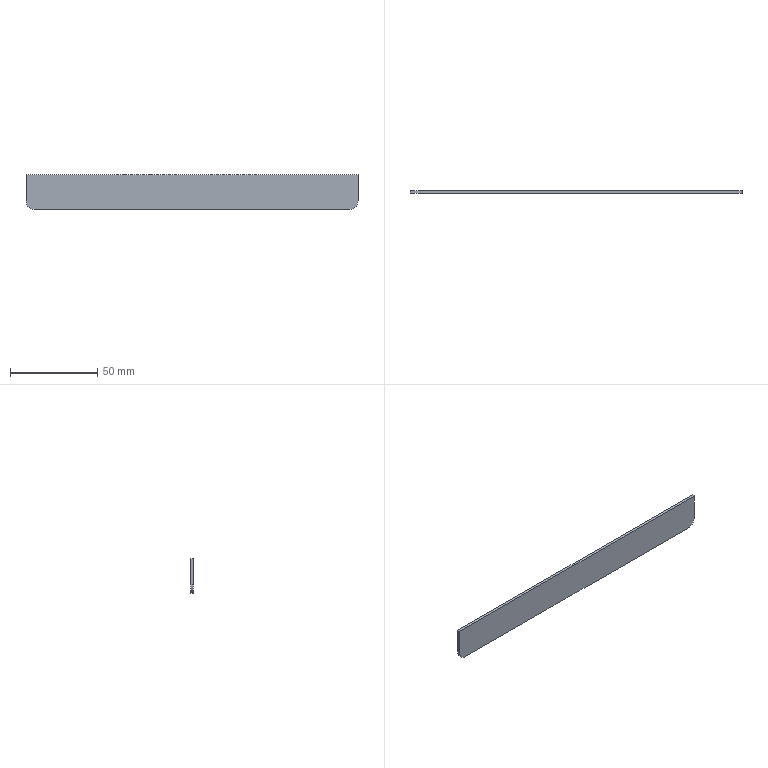Part | SolidWorks | features Extrusion 1 | 1 solid | 8 faces | box 190 x 1.6 x 20 mm | volume 6063 mm3 | plane 6 | cylinder 2 | commonest cylinder face diameters 10 x2
STEP:
#1=CARTESIAN_POINT('',(0.,0.,-15.));
#2=VERTEX_POINT('',#1);
#3=CARTESIAN_POINT('',(0.,0.,0.));
#4=VERTEX_POINT('',#3);
#5=CARTESIAN_POINT('',(0.,0.,0.));
#6=DIRECTION('',(0.,0.,1.));
#7=VECTOR('',#6,1000.);
#8=LINE('',#5,#7);
#9=EDGE_CURVE('',#2,#4,#8,.T.);
#10=ORIENTED_EDGE('',*,*,#9,.T.);
#11=CARTESIAN_POINT('',(0.,1.6,0.));
#12=VERTEX_POINT('',#11);
#13=CARTESIAN_POINT('',(0.,1.6,0.));
#14=DIRECTION('',(0.,-1.,0.));
#15=VECTOR('',#14,1000.);
#16=LINE('',#13,#15);
#17=EDGE_CURVE('',#12,#4,#16,.T.);
#18=ORIENTED_EDGE('',*,*,#17,.F.);
#19=CARTESIAN_POINT('',(0.,1.6,-15.));
#20=VERTEX_POINT('',#19);
#21=CARTESIAN_POINT('',(0.,1.6,0.));
#22=DIRECTION('',(0.,0.,1.));
#23=VECTOR('',#22,1000.);
#24=LINE('',#21,#23);
#25=EDGE_CURVE('',#20,#12,#24,.T.);
#26=ORIENTED_EDGE('',*,*,#25,.F.);
#27=CARTESIAN_POINT('',(0.,1.6,-15.));
#28=DIRECTION('',(0.,-1.,0.));
#29=VECTOR('',#28,1000.);
#30=LINE('',#27,#29);
#31=EDGE_CURVE('',#20,#2,#30,.T.);
#32=ORIENTED_EDGE('',*,*,#31,.T.);
#33=EDGE_LOOP('',(#10,#18,#26,#32));
#34=FACE_OUTER_BOUND('',#33,.T.);
#35=CARTESIAN_POINT('',(0.,1.6,0.));
#36=DIRECTION('',(1.,0.,0.));
#37=DIRECTION('',(0.,0.,-1.));
#38=AXIS2_PLACEMENT_3D('',#35,#36,#37);
#39=PLANE('',#38);
#40=ADVANCED_FACE('',(#34),#39,.F.);
#41=CARTESIAN_POINT('',(190.,0.,0.));
#42=VERTEX_POINT('',#41);
#43=CARTESIAN_POINT('',(0.,0.,0.));
#44=DIRECTION('',(1.,0.,0.));
#45=VECTOR('',#44,1000.);
#46=LINE('',#43,#45);
#47=EDGE_CURVE('',#4,#42,#46,.T.);
#48=ORIENTED_EDGE('',*,*,#47,.T.);
#49=CARTESIAN_POINT('',(190.,1.6,0.));
#50=VERTEX_POINT('',#49);
#51=CARTESIAN_POINT('',(190.,1.6,0.));
#52=DIRECTION('',(0.,-1.,0.));
#53=VECTOR('',#52,1000.);
#54=LINE('',#51,#53);
#55=EDGE_CURVE('',#50,#42,#54,.T.);
#56=ORIENTED_EDGE('',*,*,#55,.F.);
#57=CARTESIAN_POINT('',(0.,1.6,0.));
#58=DIRECTION('',(1.,0.,0.));
#59=VECTOR('',#58,1000.);
#60=LINE('',#57,#59);
#61=EDGE_CURVE('',#12,#50,#60,.T.);
#62=ORIENTED_EDGE('',*,*,#61,.F.);
#63=ORIENTED_EDGE('',*,*,#17,.T.);
#64=EDGE_LOOP('',(#48,#56,#62,#63));
#65=FACE_OUTER_BOUND('',#64,.T.);
#66=CARTESIAN_POINT('',(0.,1.6,0.));
#67=DIRECTION('',(0.,0.,-1.));
#68=DIRECTION('',(-1.,0.,0.));
#69=AXIS2_PLACEMENT_3D('',#66,#67,#68);
#70=PLANE('',#69);
#71=ADVANCED_FACE('',(#65),#70,.F.);
#72=CARTESIAN_POINT('',(190.,0.,-15.));
#73=VERTEX_POINT('',#72);
#74=CARTESIAN_POINT('',(190.,0.,0.));
#75=DIRECTION('',(0.,0.,-1.));
#76=VECTOR('',#75,1000.);
#77=LINE('',#74,#76);
#78=EDGE_CURVE('',#42,#73,#77,.T.);
#79=ORIENTED_EDGE('',*,*,#78,.T.);
#80=CARTESIAN_POINT('',(190.,1.6,-15.));
#81=VERTEX_POINT('',#80);
#82=CARTESIAN_POINT('',(190.,1.6,-15.));
#83=DIRECTION('',(0.,-1.,0.));
#84=VECTOR('',#83,1000.);
#85=LINE('',#82,#84);
#86=EDGE_CURVE('',#81,#73,#85,.T.);
#87=ORIENTED_EDGE('',*,*,#86,.F.);
#88=CARTESIAN_POINT('',(190.,1.6,0.));
#89=DIRECTION('',(0.,0.,-1.));
#90=VECTOR('',#89,1000.);
#91=LINE('',#88,#90);
#92=EDGE_CURVE('',#50,#81,#91,.T.);
#93=ORIENTED_EDGE('',*,*,#92,.F.);
#94=ORIENTED_EDGE('',*,*,#55,.T.);
#95=EDGE_LOOP('',(#79,#87,#93,#94));
#96=FACE_OUTER_BOUND('',#95,.T.);
#97=CARTESIAN_POINT('',(190.,1.6,0.));
#98=DIRECTION('',(-1.,0.,0.));
#99=DIRECTION('',(0.,0.,1.));
#100=AXIS2_PLACEMENT_3D('',#97,#98,#99);
#101=PLANE('',#100);
#102=ADVANCED_FACE('',(#96),#101,.F.);
#103=CARTESIAN_POINT('',(185.,0.,-20.));
#104=VERTEX_POINT('',#103);
#105=CARTESIAN_POINT('',(185.,0.,-15.));
#106=DIRECTION('',(0.,1.,0.));
#107=DIRECTION('',(0.,0.,-1.));
#108=AXIS2_PLACEMENT_3D('',#105,#106,#107);
#109=CIRCLE('',#108,5.);
#110=EDGE_CURVE('',#73,#104,#109,.T.);
#111=ORIENTED_EDGE('',*,*,#110,.T.);
#112=CARTESIAN_POINT('',(185.,1.6,-20.));
#113=VERTEX_POINT('',#112);
#114=CARTESIAN_POINT('',(185.,1.6,-20.));
#115=DIRECTION('',(0.,-1.,0.));
#116=VECTOR('',#115,1000.);
#117=LINE('',#114,#116);
#118=EDGE_CURVE('',#113,#104,#117,.T.);
#119=ORIENTED_EDGE('',*,*,#118,.F.);
#120=CARTESIAN_POINT('',(185.,1.6,-15.));
#121=DIRECTION('',(0.,1.,0.));
#122=DIRECTION('',(0.,0.,-1.));
#123=AXIS2_PLACEMENT_3D('',#120,#121,#122);
#124=CIRCLE('',#123,5.);
#125=EDGE_CURVE('',#81,#113,#124,.T.);
#126=ORIENTED_EDGE('',*,*,#125,.F.);
#127=ORIENTED_EDGE('',*,*,#86,.T.);
#128=EDGE_LOOP('',(#111,#119,#126,#127));
#129=FACE_OUTER_BOUND('',#128,.T.);
#130=CARTESIAN_POINT('',(185.,1.6,-15.));
#131=DIRECTION('',(0.,-1.,0.));
#132=DIRECTION('',(0.,0.,-1.));
#133=AXIS2_PLACEMENT_3D('',#130,#131,#132);
#134=CYLINDRICAL_SURFACE('',#133,5.);
#135=ADVANCED_FACE('',(#129),#134,.T.);
#136=CARTESIAN_POINT('',(5.,0.,-20.));
#137=VERTEX_POINT('',#136);
#138=CARTESIAN_POINT('',(5.,0.,-20.));
#139=DIRECTION('',(-1.,0.,0.));
#140=VECTOR('',#139,1000.);
#141=LINE('',#138,#140);
#142=EDGE_CURVE('',#104,#137,#141,.T.);
#143=ORIENTED_EDGE('',*,*,#142,.T.);
#144=CARTESIAN_POINT('',(5.,1.6,-20.));
#145=VERTEX_POINT('',#144);
#146=CARTESIAN_POINT('',(5.,1.6,-20.));
#147=DIRECTION('',(0.,-1.,0.));
#148=VECTOR('',#147,1000.);
#149=LINE('',#146,#148);
#150=EDGE_CURVE('',#145,#137,#149,.T.);
#151=ORIENTED_EDGE('',*,*,#150,.F.);
#152=CARTESIAN_POINT('',(5.,1.6,-20.));
#153=DIRECTION('',(-1.,0.,0.));
#154=VECTOR('',#153,1000.);
#155=LINE('',#152,#154);
#156=EDGE_CURVE('',#113,#145,#155,.T.);
#157=ORIENTED_EDGE('',*,*,#156,.F.);
#158=ORIENTED_EDGE('',*,*,#118,.T.);
#159=EDGE_LOOP('',(#143,#151,#157,#158));
#160=FACE_OUTER_BOUND('',#159,.T.);
#161=CARTESIAN_POINT('',(5.,1.6,-20.));
#162=DIRECTION('',(0.,0.,1.));
#163=DIRECTION('',(1.,0.,0.));
#164=AXIS2_PLACEMENT_3D('',#161,#162,#163);
#165=PLANE('',#164);
#166=ADVANCED_FACE('',(#160),#165,.F.);
#167=CARTESIAN_POINT('',(5.,0.,-15.));
#168=DIRECTION('',(0.,1.,0.));
#169=DIRECTION('',(0.,0.,-1.));
#170=AXIS2_PLACEMENT_3D('',#167,#168,#169);
#171=CIRCLE('',#170,5.);
#172=EDGE_CURVE('',#137,#2,#171,.T.);
#173=ORIENTED_EDGE('',*,*,#172,.T.);
#174=ORIENTED_EDGE('',*,*,#31,.F.);
#175=CARTESIAN_POINT('',(5.,1.6,-15.));
#176=DIRECTION('',(0.,1.,0.));
#177=DIRECTION('',(0.,0.,-1.));
#178=AXIS2_PLACEMENT_3D('',#175,#176,#177);
#179=CIRCLE('',#178,5.);
#180=EDGE_CURVE('',#145,#20,#179,.T.);
#181=ORIENTED_EDGE('',*,*,#180,.F.);
#182=ORIENTED_EDGE('',*,*,#150,.T.);
#183=EDGE_LOOP('',(#173,#174,#181,#182));
#184=FACE_OUTER_BOUND('',#183,.T.);
#185=CARTESIAN_POINT('',(5.,1.6,-15.));
#186=DIRECTION('',(0.,-1.,0.));
#187=DIRECTION('',(0.,0.,-1.));
#188=AXIS2_PLACEMENT_3D('',#185,#186,#187);
#189=CYLINDRICAL_SURFACE('',#188,5.);
#190=ADVANCED_FACE('',(#184),#189,.T.);
#191=ORIENTED_EDGE('',*,*,#25,.T.);
#192=ORIENTED_EDGE('',*,*,#61,.T.);
#193=ORIENTED_EDGE('',*,*,#92,.T.);
#194=ORIENTED_EDGE('',*,*,#125,.T.);
#195=ORIENTED_EDGE('',*,*,#156,.T.);
#196=ORIENTED_EDGE('',*,*,#180,.T.);
#197=EDGE_LOOP('',(#191,#192,#193,#194,#195,#196));
#198=FACE_OUTER_BOUND('',#197,.T.);
#199=CARTESIAN_POINT('',(5.,1.6,-15.));
#200=DIRECTION('',(0.,-1.,0.));
#201=DIRECTION('',(0.,0.,-1.));
#202=AXIS2_PLACEMENT_3D('',#199,#200,#201);
#203=PLANE('',#202);
#204=ADVANCED_FACE('',(#198),#203,.F.);
#205=ORIENTED_EDGE('',*,*,#9,.F.);
#206=ORIENTED_EDGE('',*,*,#172,.F.);
#207=ORIENTED_EDGE('',*,*,#142,.F.);
#208=ORIENTED_EDGE('',*,*,#110,.F.);
#209=ORIENTED_EDGE('',*,*,#78,.F.);
#210=ORIENTED_EDGE('',*,*,#47,.F.);
#211=EDGE_LOOP('',(#205,#206,#207,#208,#209,#210));
#212=FACE_OUTER_BOUND('',#211,.T.);
#213=CARTESIAN_POINT('',(5.,0.,-15.));
#214=DIRECTION('',(0.,-1.,0.));
#215=DIRECTION('',(0.,0.,-1.));
#216=AXIS2_PLACEMENT_3D('',#213,#214,#215);
#217=PLANE('',#216);
#218=ADVANCED_FACE('',(#212),#217,.T.);
#219=CLOSED_SHELL('',(#40,#71,#102,#135,#166,#190,#204,#218));
#220=MANIFOLD_SOLID_BREP('',#219);
#221=CARTESIAN_POINT('',(0.,0.,0.));
#222=DIRECTION('',(0.,0.,1.));
#223=DIRECTION('',(1.,0.,0.));
#224=AXIS2_PLACEMENT_3D('',#221,#222,#223);
#225=(LENGTH_UNIT()NAMED_UNIT(*)SI_UNIT(.MILLI.,.METRE.));
#226=UNCERTAINTY_MEASURE_WITH_UNIT(LENGTH_MEASURE(0.00001),#225,'','');
#227=(NAMED_UNIT(*)PLANE_ANGLE_UNIT()SI_UNIT($,.RADIAN.));
#228=(NAMED_UNIT(*)SI_UNIT($,.STERADIAN.)SOLID_ANGLE_UNIT());
#229=(GEOMETRIC_REPRESENTATION_CONTEXT(3)GLOBAL_UNCERTAINTY_ASSIGNED_CONTEXT((#226))GLOBAL_UNIT_ASSIGNED_CONTEXT((#225,#227,#228))REPRESENTATION_CONTEXT('',''));
#230=ADVANCED_BREP_SHAPE_REPRESENTATION('',(#220,#224),#229);